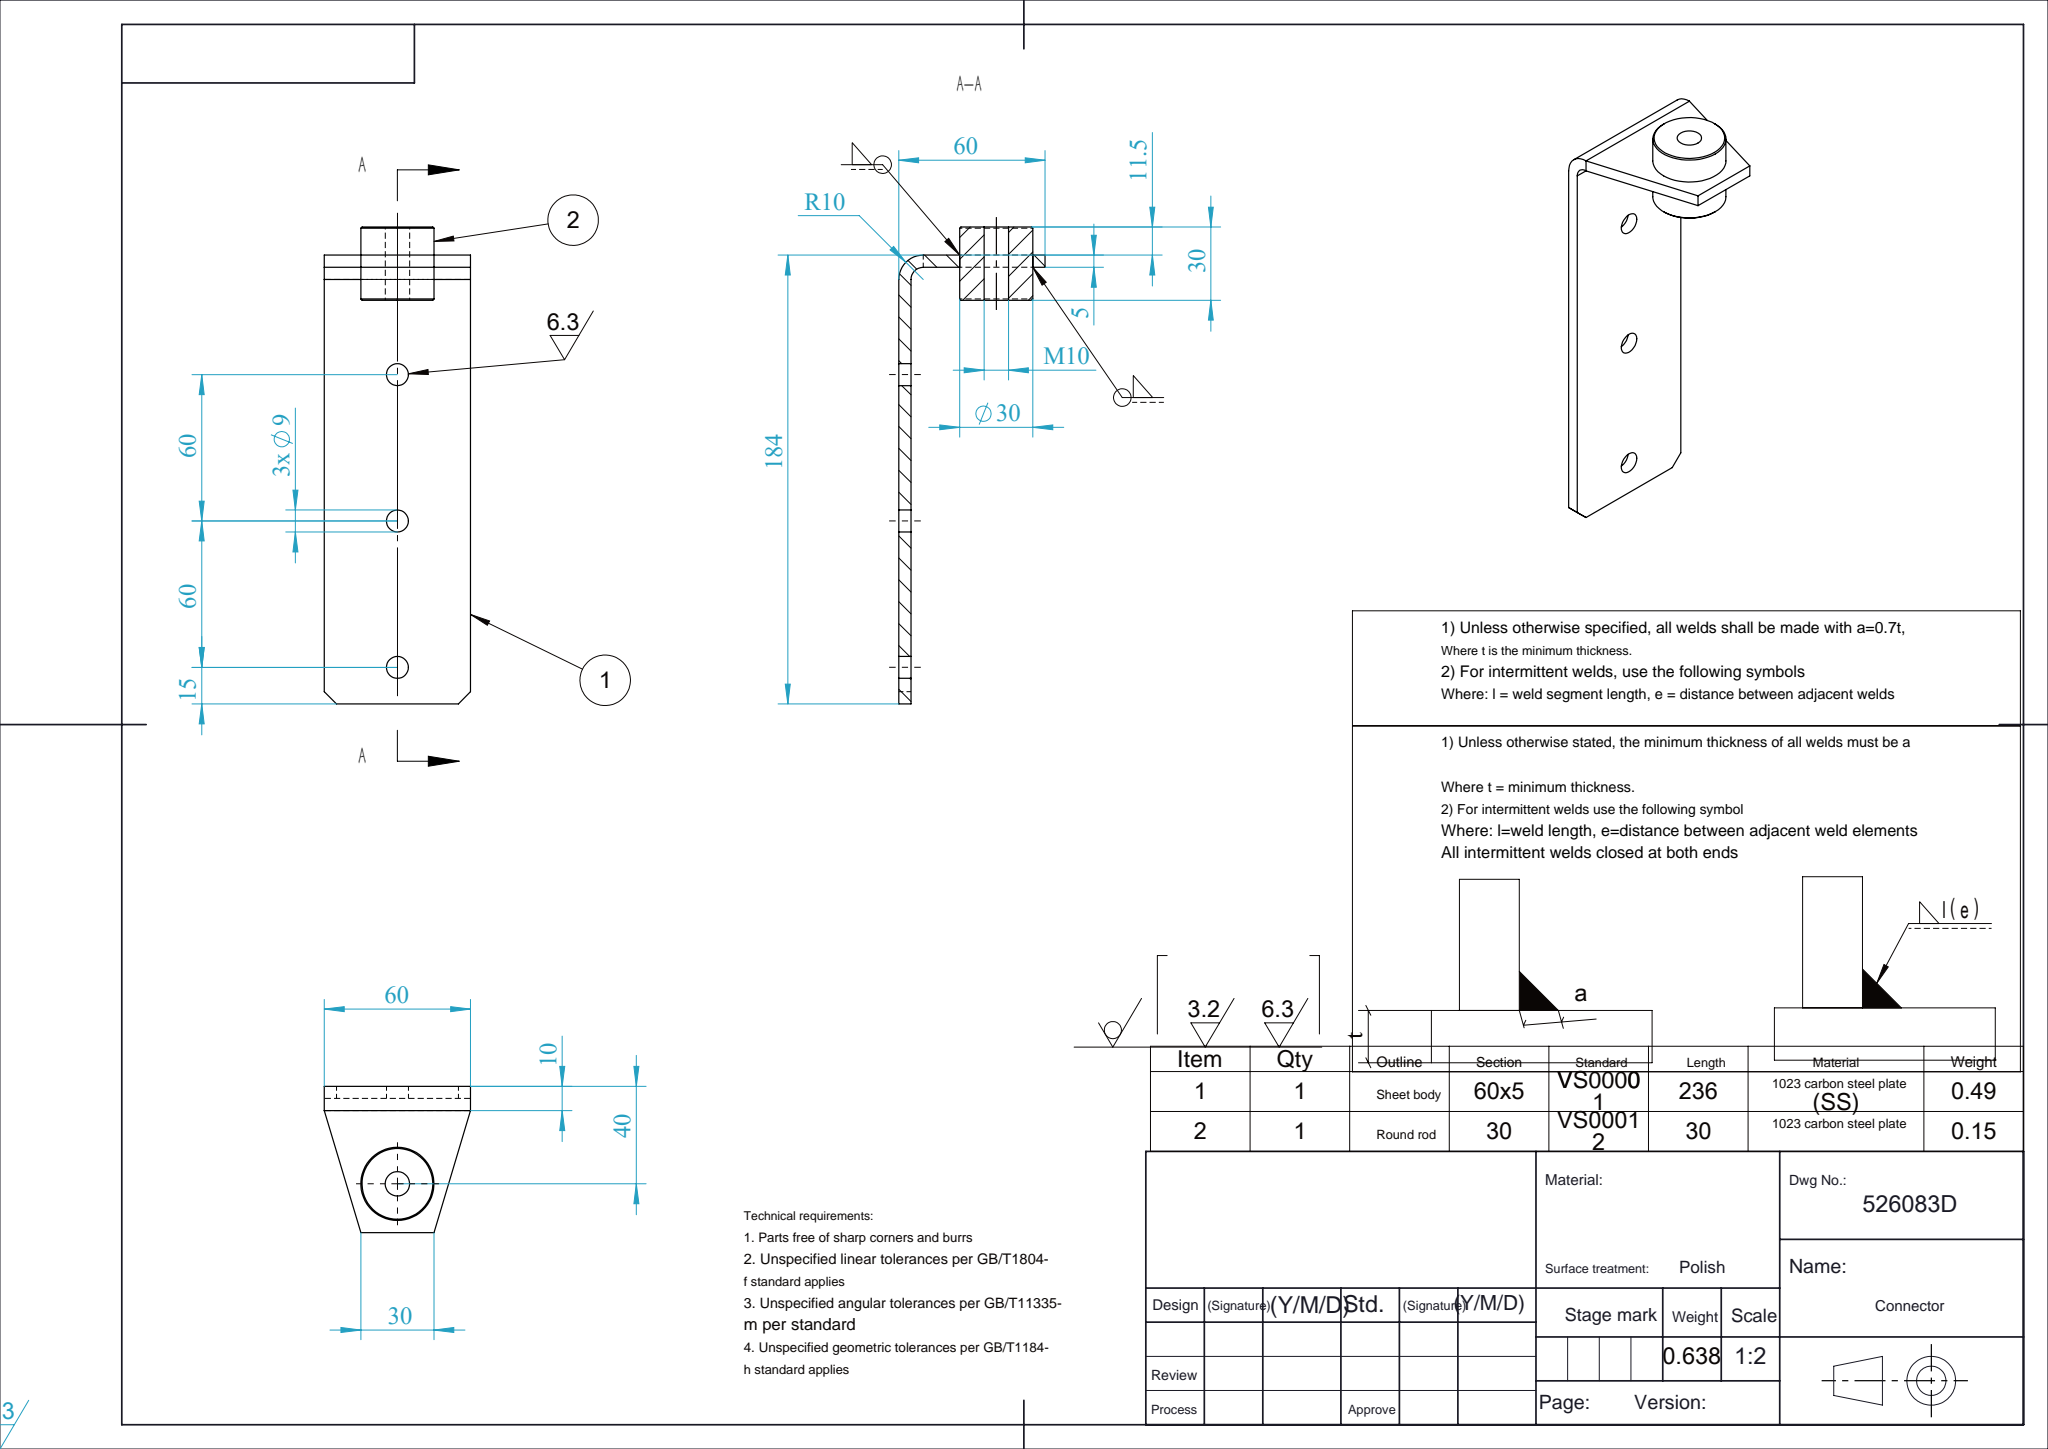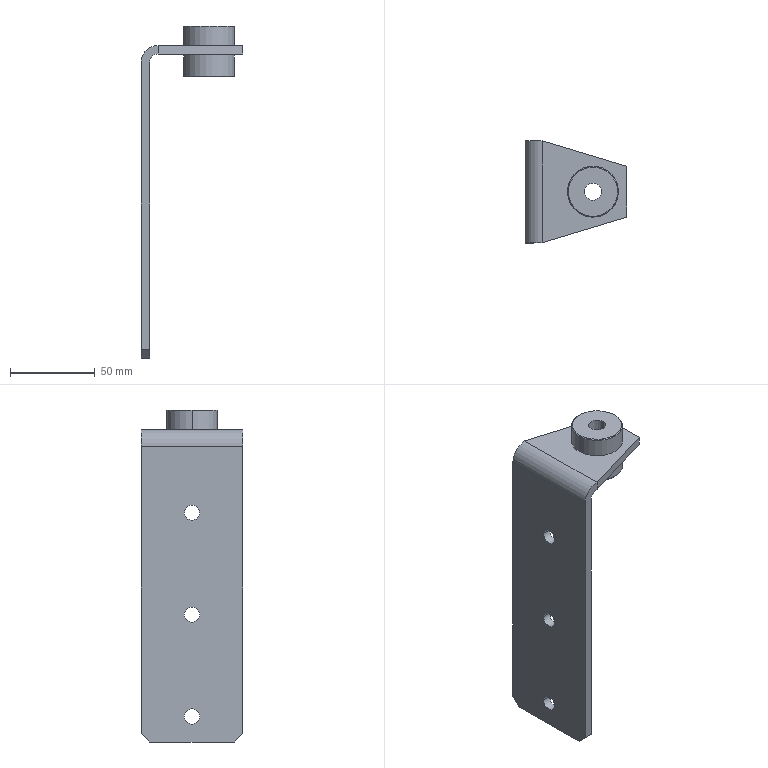Part | SolidWorks | 2 solids | 32 faces | box 60 x 60 x 195.5 mm | volume 81197 mm3 | cylinder 14 | plane 14 | cone 4 | commonest cylinder face diameters 9 x6 30 x4 10 x3 20 x1